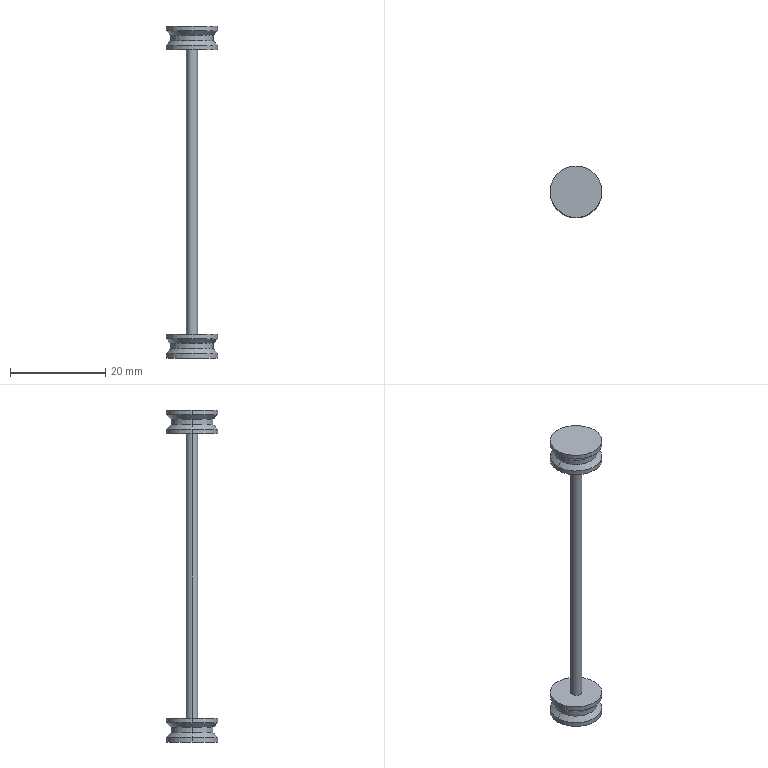Part | SolidWorks | features Extrusion 1, ICE 1, MirrorPattern 1, RefAxis 1, RevCut 1 | 1 solid | 26 faces | box 10.836 x 10.836 x 69.732 mm | volume 1053 mm3 | cylinder 14 | cone 8 | plane 4 | commonest cylinder face diameters 10.836 x8 8.853 x4 2.359 x2
STEP:
#1=CARTESIAN_POINT('',(-24.374,-6.22,-64.732));
#2=VERTEX_POINT('',#1);
#3=CARTESIAN_POINT('',(-35.209,-6.22,-64.732));
#4=VERTEX_POINT('',#3);
#5=CARTESIAN_POINT('',(-29.791,-6.22,-64.732));
#6=DIRECTION('',(0.,0.,1.));
#7=DIRECTION('',(1.,0.,0.));
#8=AXIS2_PLACEMENT_3D('',#5,#6,#7);
#9=CIRCLE('',#8,5.418);
#10=EDGE_CURVE('',#2,#4,#9,.T.);
#11=ORIENTED_EDGE('',*,*,#10,.T.);
#12=CARTESIAN_POINT('',(-35.209,-6.22,-63.774));
#13=VERTEX_POINT('',#12);
#14=CARTESIAN_POINT('',(-35.209,-6.22,-64.732));
#15=DIRECTION('',(0.,0.,1.));
#16=VECTOR('',#15,1000.);
#17=LINE('',#14,#16);
#18=EDGE_CURVE('',#4,#13,#17,.T.);
#19=ORIENTED_EDGE('',*,*,#18,.T.);
#20=CARTESIAN_POINT('',(-24.374,-6.22,-63.774));
#21=VERTEX_POINT('',#20);
#22=CARTESIAN_POINT('',(-29.791,-6.22,-63.774));
#23=DIRECTION('',(0.,0.,1.));
#24=DIRECTION('',(1.,0.,0.));
#25=AXIS2_PLACEMENT_3D('',#22,#23,#24);
#26=CIRCLE('',#25,5.418);
#27=EDGE_CURVE('',#21,#13,#26,.T.);
#28=ORIENTED_EDGE('',*,*,#27,.F.);
#29=CARTESIAN_POINT('',(-24.374,-6.22,-64.732));
#30=DIRECTION('',(0.,0.,1.));
#31=VECTOR('',#30,1000.);
#32=LINE('',#29,#31);
#33=EDGE_CURVE('',#2,#21,#32,.T.);
#34=ORIENTED_EDGE('',*,*,#33,.F.);
#35=EDGE_LOOP('',(#11,#19,#28,#34));
#36=FACE_OUTER_BOUND('',#35,.T.);
#37=CARTESIAN_POINT('',(-29.791,-6.22,-64.732));
#38=DIRECTION('',(0.,0.,1.));
#39=DIRECTION('',(1.,0.,0.));
#40=AXIS2_PLACEMENT_3D('',#37,#38,#39);
#41=CYLINDRICAL_SURFACE('',#40,5.418);
#42=ADVANCED_FACE('',(#36),#41,.T.);
#43=CARTESIAN_POINT('',(-24.374,-6.22,5.));
#44=VERTEX_POINT('',#43);
#45=CARTESIAN_POINT('',(-35.209,-6.22,5.));
#46=VERTEX_POINT('',#45);
#47=CARTESIAN_POINT('',(-29.791,-6.22,5.));
#48=DIRECTION('',(0.,0.,1.));
#49=DIRECTION('',(1.,0.,0.));
#50=AXIS2_PLACEMENT_3D('',#47,#48,#49);
#51=CIRCLE('',#50,5.418);
#52=EDGE_CURVE('',#44,#46,#51,.T.);
#53=ORIENTED_EDGE('',*,*,#52,.F.);
#54=CARTESIAN_POINT('',(-24.374,-6.22,4.042));
#55=VERTEX_POINT('',#54);
#56=CARTESIAN_POINT('',(-24.374,-6.22,5.));
#57=DIRECTION('',(0.,0.,-1.));
#58=VECTOR('',#57,1000.);
#59=LINE('',#56,#58);
#60=EDGE_CURVE('',#44,#55,#59,.T.);
#61=ORIENTED_EDGE('',*,*,#60,.T.);
#62=CARTESIAN_POINT('',(-35.209,-6.22,4.042));
#63=VERTEX_POINT('',#62);
#64=CARTESIAN_POINT('',(-29.791,-6.22,4.042));
#65=DIRECTION('',(0.,0.,1.));
#66=DIRECTION('',(1.,0.,0.));
#67=AXIS2_PLACEMENT_3D('',#64,#65,#66);
#68=CIRCLE('',#67,5.418);
#69=EDGE_CURVE('',#55,#63,#68,.T.);
#70=ORIENTED_EDGE('',*,*,#69,.T.);
#71=CARTESIAN_POINT('',(-35.209,-6.22,5.));
#72=DIRECTION('',(0.,0.,-1.));
#73=VECTOR('',#72,1000.);
#74=LINE('',#71,#73);
#75=EDGE_CURVE('',#46,#63,#74,.T.);
#76=ORIENTED_EDGE('',*,*,#75,.F.);
#77=EDGE_LOOP('',(#53,#61,#70,#76));
#78=FACE_OUTER_BOUND('',#77,.T.);
#79=CARTESIAN_POINT('',(-29.791,-6.22,5.));
#80=DIRECTION('',(0.,0.,-1.));
#81=DIRECTION('',(-1.,0.,0.));
#82=AXIS2_PLACEMENT_3D('',#79,#80,#81);
#83=CYLINDRICAL_SURFACE('',#82,5.418);
#84=ADVANCED_FACE('',(#78),#83,.T.);
#85=CARTESIAN_POINT('',(-25.365,-6.22,1.949));
#86=VERTEX_POINT('',#85);
#87=CARTESIAN_POINT('',(-34.218,-6.22,1.949));
#88=VERTEX_POINT('',#87);
#89=CARTESIAN_POINT('',(-29.791,-6.22,1.949));
#90=DIRECTION('',(0.,0.,1.));
#91=DIRECTION('',(1.,0.,0.));
#92=AXIS2_PLACEMENT_3D('',#89,#90,#91);
#93=CIRCLE('',#92,4.426);
#94=EDGE_CURVE('',#86,#88,#93,.T.);
#95=ORIENTED_EDGE('',*,*,#94,.F.);
#96=CARTESIAN_POINT('',(-24.374,-6.22,0.9579));
#97=VERTEX_POINT('',#96);
#98=CARTESIAN_POINT('',(-25.365,-6.22,1.949));
#99=DIRECTION('',(0.7071,0.,-0.7071));
#100=VECTOR('',#99,1000.);
#101=LINE('',#98,#100);
#102=EDGE_CURVE('',#86,#97,#101,.T.);
#103=ORIENTED_EDGE('',*,*,#102,.T.);
#104=CARTESIAN_POINT('',(-35.209,-6.22,0.9579));
#105=VERTEX_POINT('',#104);
#106=CARTESIAN_POINT('',(-29.791,-6.22,0.9579));
#107=DIRECTION('',(0.,0.,1.));
#108=DIRECTION('',(1.,0.,0.));
#109=AXIS2_PLACEMENT_3D('',#106,#107,#108);
#110=CIRCLE('',#109,5.418);
#111=EDGE_CURVE('',#97,#105,#110,.T.);
#112=ORIENTED_EDGE('',*,*,#111,.T.);
#113=CARTESIAN_POINT('',(-34.218,-6.22,1.949));
#114=DIRECTION('',(-0.7071,0.,-0.7071));
#115=VECTOR('',#114,1000.);
#116=LINE('',#113,#115);
#117=EDGE_CURVE('',#88,#105,#116,.T.);
#118=ORIENTED_EDGE('',*,*,#117,.F.);
#119=EDGE_LOOP('',(#95,#103,#112,#118));
#120=FACE_OUTER_BOUND('',#119,.T.);
#121=CARTESIAN_POINT('',(-29.791,-6.22,1.949));
#122=DIRECTION('',(0.,0.,-1.));
#123=DIRECTION('',(-1.,0.,0.));
#124=AXIS2_PLACEMENT_3D('',#121,#122,#123);
#125=CONICAL_SURFACE('',#124,4.426,0.7854);
#126=ADVANCED_FACE('',(#120),#125,.T.);
#127=ORIENTED_EDGE('',*,*,#94,.T.);
#128=CARTESIAN_POINT('',(-34.218,-6.22,3.051));
#129=VERTEX_POINT('',#128);
#130=CARTESIAN_POINT('',(-34.218,-6.22,5.));
#131=DIRECTION('',(0.,0.,1.));
#132=VECTOR('',#131,1000.);
#133=LINE('',#130,#132);
#134=EDGE_CURVE('',#88,#129,#133,.T.);
#135=ORIENTED_EDGE('',*,*,#134,.T.);
#136=CARTESIAN_POINT('',(-25.365,-6.22,3.051));
#137=VERTEX_POINT('',#136);
#138=CARTESIAN_POINT('',(-29.791,-6.22,3.051));
#139=DIRECTION('',(0.,0.,1.));
#140=DIRECTION('',(1.,0.,0.));
#141=AXIS2_PLACEMENT_3D('',#138,#139,#140);
#142=CIRCLE('',#141,4.426);
#143=EDGE_CURVE('',#137,#129,#142,.T.);
#144=ORIENTED_EDGE('',*,*,#143,.F.);
#145=CARTESIAN_POINT('',(-25.365,-6.22,5.));
#146=DIRECTION('',(0.,0.,1.));
#147=VECTOR('',#146,1000.);
#148=LINE('',#145,#147);
#149=EDGE_CURVE('',#86,#137,#148,.T.);
#150=ORIENTED_EDGE('',*,*,#149,.F.);
#151=EDGE_LOOP('',(#127,#135,#144,#150));
#152=FACE_OUTER_BOUND('',#151,.T.);
#153=CARTESIAN_POINT('',(-29.791,-6.22,5.));
#154=DIRECTION('',(0.,0.,1.));
#155=DIRECTION('',(1.,0.,0.));
#156=AXIS2_PLACEMENT_3D('',#153,#154,#155);
#157=CYLINDRICAL_SURFACE('',#156,4.426);
#158=ADVANCED_FACE('',(#152),#157,.T.);
#159=ORIENTED_EDGE('',*,*,#143,.T.);
#160=CARTESIAN_POINT('',(-35.209,-6.22,4.042));
#161=DIRECTION('',(-0.7071,0.,0.7071));
#162=VECTOR('',#161,1000.);
#163=LINE('',#160,#162);
#164=EDGE_CURVE('',#129,#63,#163,.T.);
#165=ORIENTED_EDGE('',*,*,#164,.T.);
#166=ORIENTED_EDGE('',*,*,#69,.F.);
#167=CARTESIAN_POINT('',(-24.374,-6.22,4.042));
#168=DIRECTION('',(0.7071,0.,0.7071));
#169=VECTOR('',#168,1000.);
#170=LINE('',#167,#169);
#171=EDGE_CURVE('',#137,#55,#170,.T.);
#172=ORIENTED_EDGE('',*,*,#171,.F.);
#173=EDGE_LOOP('',(#159,#165,#166,#172));
#174=FACE_OUTER_BOUND('',#173,.T.);
#175=CARTESIAN_POINT('',(-29.791,-6.22,4.042));
#176=DIRECTION('',(0.,0.,1.));
#177=DIRECTION('',(1.,0.,0.));
#178=AXIS2_PLACEMENT_3D('',#175,#176,#177);
#179=CONICAL_SURFACE('',#178,5.418,0.7854);
#180=ADVANCED_FACE('',(#174),#179,.T.);
#181=CARTESIAN_POINT('',(-25.365,-6.22,-62.782));
#182=VERTEX_POINT('',#181);
#183=CARTESIAN_POINT('',(-34.218,-6.22,-62.782));
#184=VERTEX_POINT('',#183);
#185=CARTESIAN_POINT('',(-29.791,-6.22,-62.782));
#186=DIRECTION('',(0.,0.,1.));
#187=DIRECTION('',(1.,0.,0.));
#188=AXIS2_PLACEMENT_3D('',#185,#186,#187);
#189=CIRCLE('',#188,4.426);
#190=EDGE_CURVE('',#182,#184,#189,.T.);
#191=ORIENTED_EDGE('',*,*,#190,.F.);
#192=CARTESIAN_POINT('',(-25.365,-6.22,-62.782));
#193=DIRECTION('',(0.7071,0.,-0.7071));
#194=VECTOR('',#193,1000.);
#195=LINE('',#192,#194);
#196=EDGE_CURVE('',#182,#21,#195,.T.);
#197=ORIENTED_EDGE('',*,*,#196,.T.);
#198=ORIENTED_EDGE('',*,*,#27,.T.);
#199=CARTESIAN_POINT('',(-34.218,-6.22,-62.782));
#200=DIRECTION('',(-0.7071,0.,-0.7071));
#201=VECTOR('',#200,1000.);
#202=LINE('',#199,#201);
#203=EDGE_CURVE('',#184,#13,#202,.T.);
#204=ORIENTED_EDGE('',*,*,#203,.F.);
#205=EDGE_LOOP('',(#191,#197,#198,#204));
#206=FACE_OUTER_BOUND('',#205,.T.);
#207=CARTESIAN_POINT('',(-29.791,-6.22,-62.782));
#208=DIRECTION('',(0.,0.,-1.));
#209=DIRECTION('',(-1.,0.,0.));
#210=AXIS2_PLACEMENT_3D('',#207,#208,#209);
#211=CONICAL_SURFACE('',#210,4.426,0.7854);
#212=ADVANCED_FACE('',(#206),#211,.T.);
#213=ORIENTED_EDGE('',*,*,#190,.T.);
#214=CARTESIAN_POINT('',(-34.218,-6.22,-61.681));
#215=VERTEX_POINT('',#214);
#216=CARTESIAN_POINT('',(-34.218,-6.22,5.));
#217=DIRECTION('',(0.,0.,1.));
#218=VECTOR('',#217,1000.);
#219=LINE('',#216,#218);
#220=EDGE_CURVE('',#184,#215,#219,.T.);
#221=ORIENTED_EDGE('',*,*,#220,.T.);
#222=CARTESIAN_POINT('',(-25.365,-6.22,-61.681));
#223=VERTEX_POINT('',#222);
#224=CARTESIAN_POINT('',(-29.791,-6.22,-61.681));
#225=DIRECTION('',(0.,0.,1.));
#226=DIRECTION('',(1.,0.,0.));
#227=AXIS2_PLACEMENT_3D('',#224,#225,#226);
#228=CIRCLE('',#227,4.426);
#229=EDGE_CURVE('',#223,#215,#228,.T.);
#230=ORIENTED_EDGE('',*,*,#229,.F.);
#231=CARTESIAN_POINT('',(-25.365,-6.22,5.));
#232=DIRECTION('',(0.,0.,1.));
#233=VECTOR('',#232,1000.);
#234=LINE('',#231,#233);
#235=EDGE_CURVE('',#182,#223,#234,.T.);
#236=ORIENTED_EDGE('',*,*,#235,.F.);
#237=EDGE_LOOP('',(#213,#221,#230,#236));
#238=FACE_OUTER_BOUND('',#237,.T.);
#239=CARTESIAN_POINT('',(-29.791,-6.22,5.));
#240=DIRECTION('',(0.,0.,1.));
#241=DIRECTION('',(1.,0.,0.));
#242=AXIS2_PLACEMENT_3D('',#239,#240,#241);
#243=CYLINDRICAL_SURFACE('',#242,4.426);
#244=ADVANCED_FACE('',(#238),#243,.T.);
#245=ORIENTED_EDGE('',*,*,#229,.T.);
#246=CARTESIAN_POINT('',(-35.209,-6.22,-60.69));
#247=VERTEX_POINT('',#246);
#248=CARTESIAN_POINT('',(-35.209,-6.22,-60.69));
#249=DIRECTION('',(-0.7071,0.,0.7071));
#250=VECTOR('',#249,1000.);
#251=LINE('',#248,#250);
#252=EDGE_CURVE('',#215,#247,#251,.T.);
#253=ORIENTED_EDGE('',*,*,#252,.T.);
#254=CARTESIAN_POINT('',(-24.374,-6.22,-60.69));
#255=VERTEX_POINT('',#254);
#256=CARTESIAN_POINT('',(-29.791,-6.22,-60.69));
#257=DIRECTION('',(0.,0.,1.));
#258=DIRECTION('',(1.,0.,0.));
#259=AXIS2_PLACEMENT_3D('',#256,#257,#258);
#260=CIRCLE('',#259,5.418);
#261=EDGE_CURVE('',#255,#247,#260,.T.);
#262=ORIENTED_EDGE('',*,*,#261,.F.);
#263=CARTESIAN_POINT('',(-24.374,-6.22,-60.69));
#264=DIRECTION('',(0.7071,0.,0.7071));
#265=VECTOR('',#264,1000.);
#266=LINE('',#263,#265);
#267=EDGE_CURVE('',#223,#255,#266,.T.);
#268=ORIENTED_EDGE('',*,*,#267,.F.);
#269=EDGE_LOOP('',(#245,#253,#262,#268));
#270=FACE_OUTER_BOUND('',#269,.T.);
#271=CARTESIAN_POINT('',(-29.791,-6.22,-60.69));
#272=DIRECTION('',(0.,0.,1.));
#273=DIRECTION('',(1.,0.,0.));
#274=AXIS2_PLACEMENT_3D('',#271,#272,#273);
#275=CONICAL_SURFACE('',#274,5.418,0.7854);
#276=ADVANCED_FACE('',(#270),#275,.T.);
#277=CARTESIAN_POINT('',(-28.612,-6.22,-59.732));
#278=VERTEX_POINT('',#277);
#279=CARTESIAN_POINT('',(-30.971,-6.22,-59.732));
#280=VERTEX_POINT('',#279);
#281=CARTESIAN_POINT('',(-29.791,-6.22,-59.732));
#282=DIRECTION('',(0.,0.,1.));
#283=DIRECTION('',(-1.,0.,0.));
#284=AXIS2_PLACEMENT_3D('',#281,#282,#283);
#285=CIRCLE('',#284,1.179);
#286=EDGE_CURVE('',#278,#280,#285,.T.);
#287=ORIENTED_EDGE('',*,*,#286,.T.);
#288=CARTESIAN_POINT('',(-30.971,-6.22,0.));
#289=VERTEX_POINT('',#288);
#290=CARTESIAN_POINT('',(-30.971,-6.22,-63.068));
#291=DIRECTION('',(0.,0.,1.));
#292=VECTOR('',#291,1000.);
#293=LINE('',#290,#292);
#294=EDGE_CURVE('',#280,#289,#293,.T.);
#295=ORIENTED_EDGE('',*,*,#294,.T.);
#296=CARTESIAN_POINT('',(-28.612,-6.22,0.));
#297=VERTEX_POINT('',#296);
#298=CARTESIAN_POINT('',(-29.791,-6.22,0.));
#299=DIRECTION('',(0.,0.,1.));
#300=DIRECTION('',(1.,0.,0.));
#301=AXIS2_PLACEMENT_3D('',#298,#299,#300);
#302=CIRCLE('',#301,1.179);
#303=EDGE_CURVE('',#297,#289,#302,.T.);
#304=ORIENTED_EDGE('',*,*,#303,.F.);
#305=CARTESIAN_POINT('',(-28.612,-6.22,-63.068));
#306=DIRECTION('',(0.,0.,1.));
#307=VECTOR('',#306,1000.);
#308=LINE('',#305,#307);
#309=EDGE_CURVE('',#278,#297,#308,.T.);
#310=ORIENTED_EDGE('',*,*,#309,.F.);
#311=EDGE_LOOP('',(#287,#295,#304,#310));
#312=FACE_OUTER_BOUND('',#311,.T.);
#313=CARTESIAN_POINT('',(-29.791,-6.22,-63.068));
#314=DIRECTION('',(0.,0.,1.));
#315=DIRECTION('',(1.,0.,0.));
#316=AXIS2_PLACEMENT_3D('',#313,#314,#315);
#317=CYLINDRICAL_SURFACE('',#316,1.179);
#318=ADVANCED_FACE('',(#312),#317,.T.);
#319=ORIENTED_EDGE('',*,*,#261,.T.);
#320=CARTESIAN_POINT('',(-35.209,-6.22,-59.732));
#321=VERTEX_POINT('',#320);
#322=CARTESIAN_POINT('',(-35.209,-6.22,-64.732));
#323=DIRECTION('',(0.,0.,1.));
#324=VECTOR('',#323,1000.);
#325=LINE('',#322,#324);
#326=EDGE_CURVE('',#247,#321,#325,.T.);
#327=ORIENTED_EDGE('',*,*,#326,.T.);
#328=CARTESIAN_POINT('',(-24.374,-6.22,-59.732));
#329=VERTEX_POINT('',#328);
#330=CARTESIAN_POINT('',(-29.791,-6.22,-59.732));
#331=DIRECTION('',(0.,0.,1.));
#332=DIRECTION('',(1.,0.,0.));
#333=AXIS2_PLACEMENT_3D('',#330,#331,#332);
#334=CIRCLE('',#333,5.418);
#335=EDGE_CURVE('',#329,#321,#334,.T.);
#336=ORIENTED_EDGE('',*,*,#335,.F.);
#337=CARTESIAN_POINT('',(-24.374,-6.22,-64.732));
#338=DIRECTION('',(0.,0.,1.));
#339=VECTOR('',#338,1000.);
#340=LINE('',#337,#339);
#341=EDGE_CURVE('',#255,#329,#340,.T.);
#342=ORIENTED_EDGE('',*,*,#341,.F.);
#343=EDGE_LOOP('',(#319,#327,#336,#342));
#344=FACE_OUTER_BOUND('',#343,.T.);
#345=CARTESIAN_POINT('',(-29.791,-6.22,-64.732));
#346=DIRECTION('',(0.,0.,1.));
#347=DIRECTION('',(1.,0.,0.));
#348=AXIS2_PLACEMENT_3D('',#345,#346,#347);
#349=CYLINDRICAL_SURFACE('',#348,5.418);
#350=ADVANCED_FACE('',(#344),#349,.T.);
#351=ORIENTED_EDGE('',*,*,#111,.F.);
#352=CARTESIAN_POINT('',(-24.374,-6.22,0.));
#353=VERTEX_POINT('',#352);
#354=CARTESIAN_POINT('',(-24.374,-6.22,5.));
#355=DIRECTION('',(0.,0.,-1.));
#356=VECTOR('',#355,1000.);
#357=LINE('',#354,#356);
#358=EDGE_CURVE('',#97,#353,#357,.T.);
#359=ORIENTED_EDGE('',*,*,#358,.T.);
#360=CARTESIAN_POINT('',(-35.209,-6.22,0.));
#361=VERTEX_POINT('',#360);
#362=CARTESIAN_POINT('',(-29.791,-6.22,0.));
#363=DIRECTION('',(0.,0.,1.));
#364=DIRECTION('',(1.,0.,0.));
#365=AXIS2_PLACEMENT_3D('',#362,#363,#364);
#366=CIRCLE('',#365,5.418);
#367=EDGE_CURVE('',#353,#361,#366,.T.);
#368=ORIENTED_EDGE('',*,*,#367,.T.);
#369=CARTESIAN_POINT('',(-35.209,-6.22,5.));
#370=DIRECTION('',(0.,0.,-1.));
#371=VECTOR('',#370,1000.);
#372=LINE('',#369,#371);
#373=EDGE_CURVE('',#105,#361,#372,.T.);
#374=ORIENTED_EDGE('',*,*,#373,.F.);
#375=EDGE_LOOP('',(#351,#359,#368,#374));
#376=FACE_OUTER_BOUND('',#375,.T.);
#377=CARTESIAN_POINT('',(-29.791,-6.22,5.));
#378=DIRECTION('',(0.,0.,-1.));
#379=DIRECTION('',(-1.,0.,0.));
#380=AXIS2_PLACEMENT_3D('',#377,#378,#379);
#381=CYLINDRICAL_SURFACE('',#380,5.418);
#382=ADVANCED_FACE('',(#376),#381,.T.);
#383=ORIENTED_EDGE('',*,*,#358,.F.);
#384=CARTESIAN_POINT('',(-29.791,-6.22,0.9579));
#385=DIRECTION('',(0.,0.,1.));
#386=DIRECTION('',(1.,0.,0.));
#387=AXIS2_PLACEMENT_3D('',#384,#385,#386);
#388=CIRCLE('',#387,5.418);
#389=EDGE_CURVE('',#105,#97,#388,.T.);
#390=ORIENTED_EDGE('',*,*,#389,.F.);
#391=ORIENTED_EDGE('',*,*,#373,.T.);
#392=CARTESIAN_POINT('',(-29.791,-6.22,0.));
#393=DIRECTION('',(0.,0.,1.));
#394=DIRECTION('',(1.,0.,0.));
#395=AXIS2_PLACEMENT_3D('',#392,#393,#394);
#396=CIRCLE('',#395,5.418);
#397=EDGE_CURVE('',#361,#353,#396,.T.);
#398=ORIENTED_EDGE('',*,*,#397,.T.);
#399=EDGE_LOOP('',(#383,#390,#391,#398));
#400=FACE_OUTER_BOUND('',#399,.T.);
#401=CARTESIAN_POINT('',(-29.791,-6.22,5.));
#402=DIRECTION('',(0.,0.,-1.));
#403=DIRECTION('',(-1.,0.,0.));
#404=AXIS2_PLACEMENT_3D('',#401,#402,#403);
#405=CYLINDRICAL_SURFACE('',#404,5.418);
#406=ADVANCED_FACE('',(#400),#405,.T.);
#407=ORIENTED_EDGE('',*,*,#326,.F.);
#408=CARTESIAN_POINT('',(-29.791,-6.22,-60.69));
#409=DIRECTION('',(0.,0.,1.));
#410=DIRECTION('',(1.,0.,0.));
#411=AXIS2_PLACEMENT_3D('',#408,#409,#410);
#412=CIRCLE('',#411,5.418);
#413=EDGE_CURVE('',#247,#255,#412,.T.);
#414=ORIENTED_EDGE('',*,*,#413,.T.);
#415=ORIENTED_EDGE('',*,*,#341,.T.);
#416=CARTESIAN_POINT('',(-29.791,-6.22,-59.732));
#417=DIRECTION('',(0.,0.,1.));
#418=DIRECTION('',(1.,0.,0.));
#419=AXIS2_PLACEMENT_3D('',#416,#417,#418);
#420=CIRCLE('',#419,5.418);
#421=EDGE_CURVE('',#321,#329,#420,.T.);
#422=ORIENTED_EDGE('',*,*,#421,.F.);
#423=EDGE_LOOP('',(#407,#414,#415,#422));
#424=FACE_OUTER_BOUND('',#423,.T.);
#425=CARTESIAN_POINT('',(-29.791,-6.22,-64.732));
#426=DIRECTION('',(0.,0.,1.));
#427=DIRECTION('',(1.,0.,0.));
#428=AXIS2_PLACEMENT_3D('',#425,#426,#427);
#429=CYLINDRICAL_SURFACE('',#428,5.418);
#430=ADVANCED_FACE('',(#424),#429,.T.);
#431=ORIENTED_EDGE('',*,*,#294,.F.);
#432=CARTESIAN_POINT('',(-29.791,-6.22,-59.732));
#433=DIRECTION('',(0.,0.,1.));
#434=DIRECTION('',(-1.,0.,0.));
#435=AXIS2_PLACEMENT_3D('',#432,#433,#434);
#436=CIRCLE('',#435,1.179);
#437=EDGE_CURVE('',#280,#278,#436,.T.);
#438=ORIENTED_EDGE('',*,*,#437,.T.);
#439=ORIENTED_EDGE('',*,*,#309,.T.);
#440=CARTESIAN_POINT('',(-29.791,-6.22,0.));
#441=DIRECTION('',(0.,0.,1.));
#442=DIRECTION('',(1.,0.,0.));
#443=AXIS2_PLACEMENT_3D('',#440,#441,#442);
#444=CIRCLE('',#443,1.179);
#445=EDGE_CURVE('',#289,#297,#444,.T.);
#446=ORIENTED_EDGE('',*,*,#445,.F.);
#447=EDGE_LOOP('',(#431,#438,#439,#446));
#448=FACE_OUTER_BOUND('',#447,.T.);
#449=CARTESIAN_POINT('',(-29.791,-6.22,-63.068));
#450=DIRECTION('',(0.,0.,1.));
#451=DIRECTION('',(1.,0.,0.));
#452=AXIS2_PLACEMENT_3D('',#449,#450,#451);
#453=CYLINDRICAL_SURFACE('',#452,1.179);
#454=ADVANCED_FACE('',(#448),#453,.T.);
#455=ORIENTED_EDGE('',*,*,#303,.T.);
#456=ORIENTED_EDGE('',*,*,#445,.T.);
#457=EDGE_LOOP('',(#455,#456));
#458=FACE_BOUND('',#457,.T.);
#459=ORIENTED_EDGE('',*,*,#397,.F.);
#460=ORIENTED_EDGE('',*,*,#367,.F.);
#461=EDGE_LOOP('',(#459,#460));
#462=FACE_OUTER_BOUND('',#461,.T.);
#463=CARTESIAN_POINT('',(-29.791,-6.22,0.));
#464=DIRECTION('',(0.,0.,1.));
#465=DIRECTION('',(1.,0.,0.));
#466=AXIS2_PLACEMENT_3D('',#463,#464,#465);
#467=PLANE('',#466);
#468=ADVANCED_FACE('',(#458,#462),#467,.F.);
#469=ORIENTED_EDGE('',*,*,#286,.F.);
#470=ORIENTED_EDGE('',*,*,#437,.F.);
#471=EDGE_LOOP('',(#469,#470));
#472=FACE_BOUND('',#471,.T.);
#473=ORIENTED_EDGE('',*,*,#335,.T.);
#474=ORIENTED_EDGE('',*,*,#421,.T.);
#475=EDGE_LOOP('',(#473,#474));
#476=FACE_OUTER_BOUND('',#475,.T.);
#477=CARTESIAN_POINT('',(-29.791,-6.22,-59.732));
#478=DIRECTION('',(0.,0.,-1.));
#479=DIRECTION('',(1.,0.,0.));
#480=AXIS2_PLACEMENT_3D('',#477,#478,#479);
#481=PLANE('',#480);
#482=ADVANCED_FACE('',(#472,#476),#481,.F.);
#483=ORIENTED_EDGE('',*,*,#252,.F.);
#484=CARTESIAN_POINT('',(-29.791,-6.22,-61.681));
#485=DIRECTION('',(0.,0.,1.));
#486=DIRECTION('',(1.,0.,0.));
#487=AXIS2_PLACEMENT_3D('',#484,#485,#486);
#488=CIRCLE('',#487,4.426);
#489=EDGE_CURVE('',#215,#223,#488,.T.);
#490=ORIENTED_EDGE('',*,*,#489,.T.);
#491=ORIENTED_EDGE('',*,*,#267,.T.);
#492=ORIENTED_EDGE('',*,*,#413,.F.);
#493=EDGE_LOOP('',(#483,#490,#491,#492));
#494=FACE_OUTER_BOUND('',#493,.T.);
#495=CARTESIAN_POINT('',(-29.791,-6.22,-60.69));
#496=DIRECTION('',(0.,0.,1.));
#497=DIRECTION('',(1.,0.,0.));
#498=AXIS2_PLACEMENT_3D('',#495,#496,#497);
#499=CONICAL_SURFACE('',#498,5.418,0.7854);
#500=ADVANCED_FACE('',(#494),#499,.T.);
#501=ORIENTED_EDGE('',*,*,#220,.F.);
#502=CARTESIAN_POINT('',(-29.791,-6.22,-62.782));
#503=DIRECTION('',(0.,0.,1.));
#504=DIRECTION('',(1.,0.,0.));
#505=AXIS2_PLACEMENT_3D('',#502,#503,#504);
#506=CIRCLE('',#505,4.426);
#507=EDGE_CURVE('',#184,#182,#506,.T.);
#508=ORIENTED_EDGE('',*,*,#507,.T.);
#509=ORIENTED_EDGE('',*,*,#235,.T.);
#510=ORIENTED_EDGE('',*,*,#489,.F.);
#511=EDGE_LOOP('',(#501,#508,#509,#510));
#512=FACE_OUTER_BOUND('',#511,.T.);
#513=CARTESIAN_POINT('',(-29.791,-6.22,5.));
#514=DIRECTION('',(0.,0.,1.));
#515=DIRECTION('',(1.,0.,0.));
#516=AXIS2_PLACEMENT_3D('',#513,#514,#515);
#517=CYLINDRICAL_SURFACE('',#516,4.426);
#518=ADVANCED_FACE('',(#512),#517,.T.);
#519=ORIENTED_EDGE('',*,*,#196,.F.);
#520=ORIENTED_EDGE('',*,*,#507,.F.);
#521=ORIENTED_EDGE('',*,*,#203,.T.);
#522=CARTESIAN_POINT('',(-29.791,-6.22,-63.774));
#523=DIRECTION('',(0.,0.,1.));
#524=DIRECTION('',(1.,0.,0.));
#525=AXIS2_PLACEMENT_3D('',#522,#523,#524);
#526=CIRCLE('',#525,5.418);
#527=EDGE_CURVE('',#13,#21,#526,.T.);
#528=ORIENTED_EDGE('',*,*,#527,.T.);
#529=EDGE_LOOP('',(#519,#520,#521,#528));
#530=FACE_OUTER_BOUND('',#529,.T.);
#531=CARTESIAN_POINT('',(-29.791,-6.22,-62.782));
#532=DIRECTION('',(0.,0.,-1.));
#533=DIRECTION('',(-1.,0.,0.));
#534=AXIS2_PLACEMENT_3D('',#531,#532,#533);
#535=CONICAL_SURFACE('',#534,4.426,0.7854);
#536=ADVANCED_FACE('',(#530),#535,.T.);
#537=ORIENTED_EDGE('',*,*,#164,.F.);
#538=CARTESIAN_POINT('',(-29.791,-6.22,3.051));
#539=DIRECTION('',(0.,0.,1.));
#540=DIRECTION('',(1.,0.,0.));
#541=AXIS2_PLACEMENT_3D('',#538,#539,#540);
#542=CIRCLE('',#541,4.426);
#543=EDGE_CURVE('',#129,#137,#542,.T.);
#544=ORIENTED_EDGE('',*,*,#543,.T.);
#545=ORIENTED_EDGE('',*,*,#171,.T.);
#546=CARTESIAN_POINT('',(-29.791,-6.22,4.042));
#547=DIRECTION('',(0.,0.,1.));
#548=DIRECTION('',(1.,0.,0.));
#549=AXIS2_PLACEMENT_3D('',#546,#547,#548);
#550=CIRCLE('',#549,5.418);
#551=EDGE_CURVE('',#63,#55,#550,.T.);
#552=ORIENTED_EDGE('',*,*,#551,.F.);
#553=EDGE_LOOP('',(#537,#544,#545,#552));
#554=FACE_OUTER_BOUND('',#553,.T.);
#555=CARTESIAN_POINT('',(-29.791,-6.22,4.042));
#556=DIRECTION('',(0.,0.,1.));
#557=DIRECTION('',(1.,0.,0.));
#558=AXIS2_PLACEMENT_3D('',#555,#556,#557);
#559=CONICAL_SURFACE('',#558,5.418,0.7854);
#560=ADVANCED_FACE('',(#554),#559,.T.);
#561=ORIENTED_EDGE('',*,*,#134,.F.);
#562=CARTESIAN_POINT('',(-29.791,-6.22,1.949));
#563=DIRECTION('',(0.,0.,1.));
#564=DIRECTION('',(1.,0.,0.));
#565=AXIS2_PLACEMENT_3D('',#562,#563,#564);
#566=CIRCLE('',#565,4.426);
#567=EDGE_CURVE('',#88,#86,#566,.T.);
#568=ORIENTED_EDGE('',*,*,#567,.T.);
#569=ORIENTED_EDGE('',*,*,#149,.T.);
#570=ORIENTED_EDGE('',*,*,#543,.F.);
#571=EDGE_LOOP('',(#561,#568,#569,#570));
#572=FACE_OUTER_BOUND('',#571,.T.);
#573=CARTESIAN_POINT('',(-29.791,-6.22,5.));
#574=DIRECTION('',(0.,0.,1.));
#575=DIRECTION('',(1.,0.,0.));
#576=AXIS2_PLACEMENT_3D('',#573,#574,#575);
#577=CYLINDRICAL_SURFACE('',#576,4.426);
#578=ADVANCED_FACE('',(#572),#577,.T.);
#579=ORIENTED_EDGE('',*,*,#102,.F.);
#580=ORIENTED_EDGE('',*,*,#567,.F.);
#581=ORIENTED_EDGE('',*,*,#117,.T.);
#582=ORIENTED_EDGE('',*,*,#389,.T.);
#583=EDGE_LOOP('',(#579,#580,#581,#582));
#584=FACE_OUTER_BOUND('',#583,.T.);
#585=CARTESIAN_POINT('',(-29.791,-6.22,1.949));
#586=DIRECTION('',(0.,0.,-1.));
#587=DIRECTION('',(-1.,0.,0.));
#588=AXIS2_PLACEMENT_3D('',#585,#586,#587);
#589=CONICAL_SURFACE('',#588,4.426,0.7854);
#590=ADVANCED_FACE('',(#584),#589,.T.);
#591=CARTESIAN_POINT('',(-29.791,-6.22,5.));
#592=DIRECTION('',(0.,0.,1.));
#593=DIRECTION('',(1.,0.,0.));
#594=AXIS2_PLACEMENT_3D('',#591,#592,#593);
#595=CIRCLE('',#594,5.418);
#596=EDGE_CURVE('',#46,#44,#595,.T.);
#597=ORIENTED_EDGE('',*,*,#596,.T.);
#598=ORIENTED_EDGE('',*,*,#52,.T.);
#599=EDGE_LOOP('',(#597,#598));
#600=FACE_OUTER_BOUND('',#599,.T.);
#601=CARTESIAN_POINT('',(-29.791,-6.22,5.));
#602=DIRECTION('',(0.,0.,1.));
#603=DIRECTION('',(1.,0.,0.));
#604=AXIS2_PLACEMENT_3D('',#601,#602,#603);
#605=PLANE('',#604);
#606=ADVANCED_FACE('',(#600),#605,.T.);
#607=ORIENTED_EDGE('',*,*,#60,.F.);
#608=ORIENTED_EDGE('',*,*,#596,.F.);
#609=ORIENTED_EDGE('',*,*,#75,.T.);
#610=ORIENTED_EDGE('',*,*,#551,.T.);
#611=EDGE_LOOP('',(#607,#608,#609,#610));
#612=FACE_OUTER_BOUND('',#611,.T.);
#613=CARTESIAN_POINT('',(-29.791,-6.22,5.));
#614=DIRECTION('',(0.,0.,-1.));
#615=DIRECTION('',(-1.,0.,0.));
#616=AXIS2_PLACEMENT_3D('',#613,#614,#615);
#617=CYLINDRICAL_SURFACE('',#616,5.418);
#618=ADVANCED_FACE('',(#612),#617,.T.);
#619=ORIENTED_EDGE('',*,*,#10,.F.);
#620=CARTESIAN_POINT('',(-29.791,-6.22,-64.732));
#621=DIRECTION('',(0.,0.,1.));
#622=DIRECTION('',(1.,0.,0.));
#623=AXIS2_PLACEMENT_3D('',#620,#621,#622);
#624=CIRCLE('',#623,5.418);
#625=EDGE_CURVE('',#4,#2,#624,.T.);
#626=ORIENTED_EDGE('',*,*,#625,.F.);
#627=EDGE_LOOP('',(#619,#626));
#628=FACE_OUTER_BOUND('',#627,.T.);
#629=CARTESIAN_POINT('',(-29.791,-6.22,-64.732));
#630=DIRECTION('',(0.,0.,-1.));
#631=DIRECTION('',(1.,0.,0.));
#632=AXIS2_PLACEMENT_3D('',#629,#630,#631);
#633=PLANE('',#632);
#634=ADVANCED_FACE('',(#628),#633,.T.);
#635=ORIENTED_EDGE('',*,*,#18,.F.);
#636=ORIENTED_EDGE('',*,*,#625,.T.);
#637=ORIENTED_EDGE('',*,*,#33,.T.);
#638=ORIENTED_EDGE('',*,*,#527,.F.);
#639=EDGE_LOOP('',(#635,#636,#637,#638));
#640=FACE_OUTER_BOUND('',#639,.T.);
#641=CARTESIAN_POINT('',(-29.791,-6.22,-64.732));
#642=DIRECTION('',(0.,0.,1.));
#643=DIRECTION('',(1.,0.,0.));
#644=AXIS2_PLACEMENT_3D('',#641,#642,#643);
#645=CYLINDRICAL_SURFACE('',#644,5.418);
#646=ADVANCED_FACE('',(#640),#645,.T.);
#647=CLOSED_SHELL('',(#42,#84,#126,#158,#180,#212,#244,#276,#318,#350,#382,#406,#430,#454,#468,#482,#500,#518,#536,#560,#578,#590,#606,#618,#634,#646));
#648=MANIFOLD_SOLID_BREP('',#647);
#649=CARTESIAN_POINT('',(0.,0.,0.));
#650=DIRECTION('',(0.,0.,1.));
#651=DIRECTION('',(1.,0.,0.));
#652=AXIS2_PLACEMENT_3D('',#649,#650,#651);
#653=(LENGTH_UNIT()NAMED_UNIT(*)SI_UNIT(.MILLI.,.METRE.));
#654=UNCERTAINTY_MEASURE_WITH_UNIT(LENGTH_MEASURE(0.00001),#653,'','');
#655=(NAMED_UNIT(*)PLANE_ANGLE_UNIT()SI_UNIT($,.RADIAN.));
#656=(NAMED_UNIT(*)SI_UNIT($,.STERADIAN.)SOLID_ANGLE_UNIT());
#657=(GEOMETRIC_REPRESENTATION_CONTEXT(3)GLOBAL_UNCERTAINTY_ASSIGNED_CONTEXT((#654))GLOBAL_UNIT_ASSIGNED_CONTEXT((#653,#655,#656))REPRESENTATION_CONTEXT('',''));
#658=ADVANCED_BREP_SHAPE_REPRESENTATION('',(#648,#652),#657);